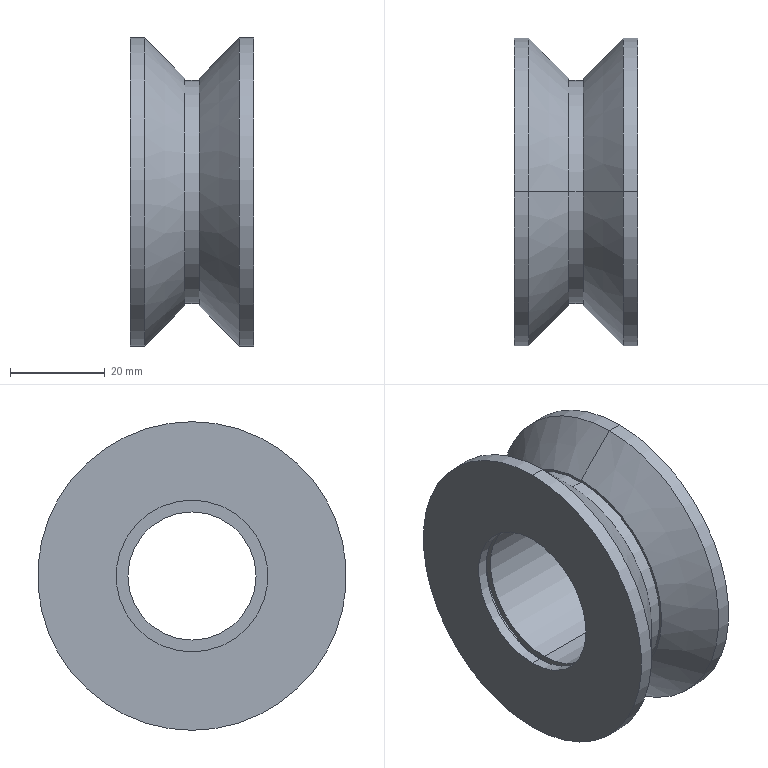Part | STEP file | X77-03304 | 1 solid | 25 faces | box 26 x 65 x 65 mm | volume 47550 mm3 | cylinder 14 | plane 7 | cone 4 | commonest cylinder face diameters 32 x4 65 x4 27 x2 34.6 x2 47 x2
STEP:
#1=CARTESIAN_POINT('',(10.752,77.79,23.5));
#2=VERTEX_POINT('',#1);
#3=CARTESIAN_POINT('',(10.752,77.79,-23.5));
#4=VERTEX_POINT('',#3);
#5=CARTESIAN_POINT('',(10.752,77.79,0.));
#6=DIRECTION('',(-1.,0.,0.));
#7=DIRECTION('',(0.,0.,1.));
#8=AXIS2_PLACEMENT_3D('',#5,#6,#7);
#9=CIRCLE('',#8,23.5);
#10=EDGE_CURVE('',#2,#4,#9,.T.);
#11=ORIENTED_EDGE('',*,*,#10,.T.);
#12=CARTESIAN_POINT('',(7.752,77.79,-23.5));
#13=VERTEX_POINT('',#12);
#14=CARTESIAN_POINT('',(-1000.,77.79,-23.5));
#15=DIRECTION('',(-1.,0.,0.));
#16=VECTOR('',#15,1000.);
#17=LINE('',#14,#16);
#18=EDGE_CURVE('',#4,#13,#17,.T.);
#19=ORIENTED_EDGE('',*,*,#18,.T.);
#20=CARTESIAN_POINT('',(7.752,77.79,23.5));
#21=VERTEX_POINT('',#20);
#22=CARTESIAN_POINT('',(7.752,77.79,0.));
#23=DIRECTION('',(-1.,0.,0.));
#24=DIRECTION('',(0.,0.,1.));
#25=AXIS2_PLACEMENT_3D('',#22,#23,#24);
#26=CIRCLE('',#25,23.5);
#27=EDGE_CURVE('',#21,#13,#26,.T.);
#28=ORIENTED_EDGE('',*,*,#27,.F.);
#29=CARTESIAN_POINT('',(-1000.,77.79,23.5));
#30=DIRECTION('',(-1.,0.,0.));
#31=VECTOR('',#30,1000.);
#32=LINE('',#29,#31);
#33=EDGE_CURVE('',#2,#21,#32,.T.);
#34=ORIENTED_EDGE('',*,*,#33,.F.);
#35=EDGE_LOOP('',(#11,#19,#28,#34));
#36=FACE_OUTER_BOUND('',#35,.T.);
#37=CARTESIAN_POINT('',(-1000.,77.79,0.));
#38=DIRECTION('',(-1.,0.,0.));
#39=DIRECTION('',(0.,0.,1.));
#40=AXIS2_PLACEMENT_3D('',#37,#38,#39);
#41=CYLINDRICAL_SURFACE('',#40,23.5);
#42=ADVANCED_FACE('',(#36),#41,.T.);
#43=CARTESIAN_POINT('',(7.752,77.79,24.));
#44=VERTEX_POINT('',#43);
#45=CARTESIAN_POINT('',(7.752,77.79,-24.));
#46=VERTEX_POINT('',#45);
#47=CARTESIAN_POINT('',(7.752,77.79,0.));
#48=DIRECTION('',(-1.,0.,0.));
#49=DIRECTION('',(0.,0.,1.));
#50=AXIS2_PLACEMENT_3D('',#47,#48,#49);
#51=CIRCLE('',#50,24.);
#52=EDGE_CURVE('',#44,#46,#51,.T.);
#53=ORIENTED_EDGE('',*,*,#52,.T.);
#54=CARTESIAN_POINT('',(-0.7476,77.79,-32.5));
#55=VERTEX_POINT('',#54);
#56=CARTESIAN_POINT('',(7.752,77.79,-24.));
#57=DIRECTION('',(-0.7071,0.,-0.7071));
#58=VECTOR('',#57,1000.);
#59=LINE('',#56,#58);
#60=EDGE_CURVE('',#46,#55,#59,.T.);
#61=ORIENTED_EDGE('',*,*,#60,.T.);
#62=CARTESIAN_POINT('',(-0.7476,77.79,32.5));
#63=VERTEX_POINT('',#62);
#64=CARTESIAN_POINT('',(-0.7476,77.79,0.));
#65=DIRECTION('',(-1.,0.,0.));
#66=DIRECTION('',(0.,0.,1.));
#67=AXIS2_PLACEMENT_3D('',#64,#65,#66);
#68=CIRCLE('',#67,32.5);
#69=EDGE_CURVE('',#63,#55,#68,.T.);
#70=ORIENTED_EDGE('',*,*,#69,.F.);
#71=CARTESIAN_POINT('',(7.752,77.79,24.));
#72=DIRECTION('',(-0.7071,0.,0.7071));
#73=VECTOR('',#72,1000.);
#74=LINE('',#71,#73);
#75=EDGE_CURVE('',#44,#63,#74,.T.);
#76=ORIENTED_EDGE('',*,*,#75,.F.);
#77=EDGE_LOOP('',(#53,#61,#70,#76));
#78=FACE_OUTER_BOUND('',#77,.T.);
#79=CARTESIAN_POINT('',(7.752,77.79,0.));
#80=DIRECTION('',(-1.,0.,0.));
#81=DIRECTION('',(0.,0.,1.));
#82=AXIS2_PLACEMENT_3D('',#79,#80,#81);
#83=CONICAL_SURFACE('',#82,24.,0.7854);
#84=ADVANCED_FACE('',(#78),#83,.T.);
#85=ORIENTED_EDGE('',*,*,#69,.T.);
#86=CARTESIAN_POINT('',(-3.748,77.79,-32.5));
#87=VERTEX_POINT('',#86);
#88=CARTESIAN_POINT('',(-1000.,77.79,-32.5));
#89=DIRECTION('',(-1.,0.,0.));
#90=VECTOR('',#89,1000.);
#91=LINE('',#88,#90);
#92=EDGE_CURVE('',#55,#87,#91,.T.);
#93=ORIENTED_EDGE('',*,*,#92,.T.);
#94=CARTESIAN_POINT('',(-3.748,77.79,32.5));
#95=VERTEX_POINT('',#94);
#96=CARTESIAN_POINT('',(-3.748,77.79,0.));
#97=DIRECTION('',(-1.,0.,0.));
#98=DIRECTION('',(0.,0.,1.));
#99=AXIS2_PLACEMENT_3D('',#96,#97,#98);
#100=CIRCLE('',#99,32.5);
#101=EDGE_CURVE('',#95,#87,#100,.T.);
#102=ORIENTED_EDGE('',*,*,#101,.F.);
#103=CARTESIAN_POINT('',(-1000.,77.79,32.5));
#104=DIRECTION('',(-1.,0.,0.));
#105=VECTOR('',#104,1000.);
#106=LINE('',#103,#105);
#107=EDGE_CURVE('',#63,#95,#106,.T.);
#108=ORIENTED_EDGE('',*,*,#107,.F.);
#109=EDGE_LOOP('',(#85,#93,#102,#108));
#110=FACE_OUTER_BOUND('',#109,.T.);
#111=CARTESIAN_POINT('',(-1000.,77.79,0.));
#112=DIRECTION('',(-1.,0.,0.));
#113=DIRECTION('',(0.,0.,1.));
#114=AXIS2_PLACEMENT_3D('',#111,#112,#113);
#115=CYLINDRICAL_SURFACE('',#114,32.5);
#116=ADVANCED_FACE('',(#110),#115,.T.);
#117=CARTESIAN_POINT('',(-1.548,77.79,-16.));
#118=VERTEX_POINT('',#117);
#119=CARTESIAN_POINT('',(-1.548,77.79,16.));
#120=VERTEX_POINT('',#119);
#121=CARTESIAN_POINT('',(-1.548,77.79,0.));
#122=DIRECTION('',(-1.,0.,0.));
#123=DIRECTION('',(0.,0.,1.));
#124=AXIS2_PLACEMENT_3D('',#121,#122,#123);
#125=CIRCLE('',#124,16.);
#126=EDGE_CURVE('',#118,#120,#125,.T.);
#127=ORIENTED_EDGE('',*,*,#126,.F.);
#128=CARTESIAN_POINT('',(-3.748,77.79,-16.));
#129=VERTEX_POINT('',#128);
#130=CARTESIAN_POINT('',(-1000.,77.79,-16.));
#131=DIRECTION('',(-1.,0.,0.));
#132=VECTOR('',#131,1000.);
#133=LINE('',#130,#132);
#134=EDGE_CURVE('',#118,#129,#133,.T.);
#135=ORIENTED_EDGE('',*,*,#134,.T.);
#136=CARTESIAN_POINT('',(-3.748,77.79,16.));
#137=VERTEX_POINT('',#136);
#138=CARTESIAN_POINT('',(-3.748,77.79,0.));
#139=DIRECTION('',(-1.,0.,0.));
#140=DIRECTION('',(0.,0.,1.));
#141=AXIS2_PLACEMENT_3D('',#138,#139,#140);
#142=CIRCLE('',#141,16.);
#143=EDGE_CURVE('',#129,#137,#142,.T.);
#144=ORIENTED_EDGE('',*,*,#143,.T.);
#145=CARTESIAN_POINT('',(-1000.,77.79,16.));
#146=DIRECTION('',(-1.,0.,0.));
#147=VECTOR('',#146,1000.);
#148=LINE('',#145,#147);
#149=EDGE_CURVE('',#120,#137,#148,.T.);
#150=ORIENTED_EDGE('',*,*,#149,.F.);
#151=EDGE_LOOP('',(#127,#135,#144,#150));
#152=FACE_OUTER_BOUND('',#151,.T.);
#153=CARTESIAN_POINT('',(-1000.,77.79,0.));
#154=DIRECTION('',(-1.,0.,0.));
#155=DIRECTION('',(0.,0.,1.));
#156=AXIS2_PLACEMENT_3D('',#153,#154,#155);
#157=CYLINDRICAL_SURFACE('',#156,16.);
#158=ADVANCED_FACE('',(#152),#157,.F.);
#159=CARTESIAN_POINT('',(-0.2476,77.79,-17.3));
#160=VERTEX_POINT('',#159);
#161=CARTESIAN_POINT('',(-0.2476,77.79,17.3));
#162=VERTEX_POINT('',#161);
#163=CARTESIAN_POINT('',(-0.2476,77.79,0.));
#164=DIRECTION('',(-1.,0.,0.));
#165=DIRECTION('',(0.,0.,1.));
#166=AXIS2_PLACEMENT_3D('',#163,#164,#165);
#167=CIRCLE('',#166,17.3);
#168=EDGE_CURVE('',#160,#162,#167,.T.);
#169=ORIENTED_EDGE('',*,*,#168,.F.);
#170=CARTESIAN_POINT('',(-1.548,77.79,-17.3));
#171=VERTEX_POINT('',#170);
#172=CARTESIAN_POINT('',(-1000.,77.79,-17.3));
#173=DIRECTION('',(-1.,0.,0.));
#174=VECTOR('',#173,1000.);
#175=LINE('',#172,#174);
#176=EDGE_CURVE('',#160,#171,#175,.T.);
#177=ORIENTED_EDGE('',*,*,#176,.T.);
#178=CARTESIAN_POINT('',(-1.548,77.79,17.3));
#179=VERTEX_POINT('',#178);
#180=CARTESIAN_POINT('',(-1.548,77.79,0.));
#181=DIRECTION('',(-1.,0.,0.));
#182=DIRECTION('',(0.,0.,1.));
#183=AXIS2_PLACEMENT_3D('',#180,#181,#182);
#184=CIRCLE('',#183,17.3);
#185=EDGE_CURVE('',#171,#179,#184,.T.);
#186=ORIENTED_EDGE('',*,*,#185,.T.);
#187=CARTESIAN_POINT('',(-1000.,77.79,17.3));
#188=DIRECTION('',(-1.,0.,0.));
#189=VECTOR('',#188,1000.);
#190=LINE('',#187,#189);
#191=EDGE_CURVE('',#162,#179,#190,.T.);
#192=ORIENTED_EDGE('',*,*,#191,.F.);
#193=EDGE_LOOP('',(#169,#177,#186,#192));
#194=FACE_OUTER_BOUND('',#193,.T.);
#195=CARTESIAN_POINT('',(-1000.,77.79,0.));
#196=DIRECTION('',(-1.,0.,0.));
#197=DIRECTION('',(0.,0.,1.));
#198=AXIS2_PLACEMENT_3D('',#195,#196,#197);
#199=CYLINDRICAL_SURFACE('',#198,17.3);
#200=ADVANCED_FACE('',(#194),#199,.F.);
#201=CARTESIAN_POINT('',(19.752,77.79,-16.));
#202=VERTEX_POINT('',#201);
#203=CARTESIAN_POINT('',(19.752,77.79,16.));
#204=VERTEX_POINT('',#203);
#205=CARTESIAN_POINT('',(19.752,77.79,0.));
#206=DIRECTION('',(-1.,0.,0.));
#207=DIRECTION('',(0.,0.,1.));
#208=AXIS2_PLACEMENT_3D('',#205,#206,#207);
#209=CIRCLE('',#208,16.);
#210=EDGE_CURVE('',#202,#204,#209,.T.);
#211=ORIENTED_EDGE('',*,*,#210,.F.);
#212=CARTESIAN_POINT('',(-0.2476,77.79,-16.));
#213=VERTEX_POINT('',#212);
#214=CARTESIAN_POINT('',(-1000.,77.79,-16.));
#215=DIRECTION('',(-1.,0.,0.));
#216=VECTOR('',#215,1000.);
#217=LINE('',#214,#216);
#218=EDGE_CURVE('',#202,#213,#217,.T.);
#219=ORIENTED_EDGE('',*,*,#218,.T.);
#220=CARTESIAN_POINT('',(-0.2476,77.79,16.));
#221=VERTEX_POINT('',#220);
#222=CARTESIAN_POINT('',(-0.2476,77.79,0.));
#223=DIRECTION('',(-1.,0.,0.));
#224=DIRECTION('',(0.,0.,1.));
#225=AXIS2_PLACEMENT_3D('',#222,#223,#224);
#226=CIRCLE('',#225,16.);
#227=EDGE_CURVE('',#213,#221,#226,.T.);
#228=ORIENTED_EDGE('',*,*,#227,.T.);
#229=CARTESIAN_POINT('',(-1000.,77.79,16.));
#230=DIRECTION('',(-1.,0.,0.));
#231=VECTOR('',#230,1000.);
#232=LINE('',#229,#231);
#233=EDGE_CURVE('',#204,#221,#232,.T.);
#234=ORIENTED_EDGE('',*,*,#233,.F.);
#235=EDGE_LOOP('',(#211,#219,#228,#234));
#236=FACE_OUTER_BOUND('',#235,.T.);
#237=CARTESIAN_POINT('',(-1000.,77.79,0.));
#238=DIRECTION('',(-1.,0.,0.));
#239=DIRECTION('',(0.,0.,1.));
#240=AXIS2_PLACEMENT_3D('',#237,#238,#239);
#241=CYLINDRICAL_SURFACE('',#240,16.);
#242=ADVANCED_FACE('',(#236),#241,.F.);
#243=CARTESIAN_POINT('',(22.252,77.79,-13.5));
#244=VERTEX_POINT('',#243);
#245=CARTESIAN_POINT('',(22.252,77.79,13.5));
#246=VERTEX_POINT('',#245);
#247=CARTESIAN_POINT('',(22.252,77.79,0.));
#248=DIRECTION('',(-1.,0.,0.));
#249=DIRECTION('',(0.,0.,1.));
#250=AXIS2_PLACEMENT_3D('',#247,#248,#249);
#251=CIRCLE('',#250,13.5);
#252=EDGE_CURVE('',#244,#246,#251,.T.);
#253=ORIENTED_EDGE('',*,*,#252,.F.);
#254=CARTESIAN_POINT('',(19.752,77.79,-13.5));
#255=VERTEX_POINT('',#254);
#256=CARTESIAN_POINT('',(-1000.,77.79,-13.5));
#257=DIRECTION('',(-1.,0.,0.));
#258=VECTOR('',#257,1000.);
#259=LINE('',#256,#258);
#260=EDGE_CURVE('',#244,#255,#259,.T.);
#261=ORIENTED_EDGE('',*,*,#260,.T.);
#262=CARTESIAN_POINT('',(19.752,77.79,13.5));
#263=VERTEX_POINT('',#262);
#264=CARTESIAN_POINT('',(19.752,77.79,0.));
#265=DIRECTION('',(-1.,0.,0.));
#266=DIRECTION('',(0.,0.,1.));
#267=AXIS2_PLACEMENT_3D('',#264,#265,#266);
#268=CIRCLE('',#267,13.5);
#269=EDGE_CURVE('',#255,#263,#268,.T.);
#270=ORIENTED_EDGE('',*,*,#269,.T.);
#271=CARTESIAN_POINT('',(-1000.,77.79,13.5));
#272=DIRECTION('',(-1.,0.,0.));
#273=VECTOR('',#272,1000.);
#274=LINE('',#271,#273);
#275=EDGE_CURVE('',#246,#263,#274,.T.);
#276=ORIENTED_EDGE('',*,*,#275,.F.);
#277=EDGE_LOOP('',(#253,#261,#270,#276));
#278=FACE_OUTER_BOUND('',#277,.T.);
#279=CARTESIAN_POINT('',(-1000.,77.79,0.));
#280=DIRECTION('',(-1.,0.,0.));
#281=DIRECTION('',(0.,0.,1.));
#282=AXIS2_PLACEMENT_3D('',#279,#280,#281);
#283=CYLINDRICAL_SURFACE('',#282,13.5);
#284=ADVANCED_FACE('',(#278),#283,.F.);
#285=CARTESIAN_POINT('',(22.252,77.79,32.5));
#286=VERTEX_POINT('',#285);
#287=CARTESIAN_POINT('',(22.252,77.79,-32.5));
#288=VERTEX_POINT('',#287);
#289=CARTESIAN_POINT('',(22.252,77.79,0.));
#290=DIRECTION('',(-1.,0.,0.));
#291=DIRECTION('',(0.,0.,1.));
#292=AXIS2_PLACEMENT_3D('',#289,#290,#291);
#293=CIRCLE('',#292,32.5);
#294=EDGE_CURVE('',#286,#288,#293,.T.);
#295=ORIENTED_EDGE('',*,*,#294,.T.);
#296=CARTESIAN_POINT('',(19.252,77.79,-32.5));
#297=VERTEX_POINT('',#296);
#298=CARTESIAN_POINT('',(-1000.,77.79,-32.5));
#299=DIRECTION('',(-1.,0.,0.));
#300=VECTOR('',#299,1000.);
#301=LINE('',#298,#300);
#302=EDGE_CURVE('',#288,#297,#301,.T.);
#303=ORIENTED_EDGE('',*,*,#302,.T.);
#304=CARTESIAN_POINT('',(19.252,77.79,32.5));
#305=VERTEX_POINT('',#304);
#306=CARTESIAN_POINT('',(19.252,77.79,0.));
#307=DIRECTION('',(-1.,0.,0.));
#308=DIRECTION('',(0.,0.,1.));
#309=AXIS2_PLACEMENT_3D('',#306,#307,#308);
#310=CIRCLE('',#309,32.5);
#311=EDGE_CURVE('',#305,#297,#310,.T.);
#312=ORIENTED_EDGE('',*,*,#311,.F.);
#313=CARTESIAN_POINT('',(-1000.,77.79,32.5));
#314=DIRECTION('',(-1.,0.,0.));
#315=VECTOR('',#314,1000.);
#316=LINE('',#313,#315);
#317=EDGE_CURVE('',#286,#305,#316,.T.);
#318=ORIENTED_EDGE('',*,*,#317,.F.);
#319=EDGE_LOOP('',(#295,#303,#312,#318));
#320=FACE_OUTER_BOUND('',#319,.T.);
#321=CARTESIAN_POINT('',(-1000.,77.79,0.));
#322=DIRECTION('',(-1.,0.,0.));
#323=DIRECTION('',(0.,0.,1.));
#324=AXIS2_PLACEMENT_3D('',#321,#322,#323);
#325=CYLINDRICAL_SURFACE('',#324,32.5);
#326=ADVANCED_FACE('',(#320),#325,.T.);
#327=CARTESIAN_POINT('',(10.752,77.79,24.));
#328=VERTEX_POINT('',#327);
#329=CARTESIAN_POINT('',(10.752,77.79,-24.));
#330=VERTEX_POINT('',#329);
#331=CARTESIAN_POINT('',(10.752,77.79,0.));
#332=DIRECTION('',(-1.,0.,0.));
#333=DIRECTION('',(0.,0.,1.));
#334=AXIS2_PLACEMENT_3D('',#331,#332,#333);
#335=CIRCLE('',#334,24.);
#336=EDGE_CURVE('',#328,#330,#335,.T.);
#337=ORIENTED_EDGE('',*,*,#336,.F.);
#338=CARTESIAN_POINT('',(19.252,77.79,32.5));
#339=DIRECTION('',(0.7071,0.,0.7071));
#340=VECTOR('',#339,1000.);
#341=LINE('',#338,#340);
#342=EDGE_CURVE('',#328,#305,#341,.T.);
#343=ORIENTED_EDGE('',*,*,#342,.T.);
#344=ORIENTED_EDGE('',*,*,#311,.T.);
#345=CARTESIAN_POINT('',(19.252,77.79,-32.5));
#346=DIRECTION('',(0.7071,0.,-0.7071));
#347=VECTOR('',#346,1000.);
#348=LINE('',#345,#347);
#349=EDGE_CURVE('',#330,#297,#348,.T.);
#350=ORIENTED_EDGE('',*,*,#349,.F.);
#351=EDGE_LOOP('',(#337,#343,#344,#350));
#352=FACE_OUTER_BOUND('',#351,.T.);
#353=CARTESIAN_POINT('',(19.252,77.79,0.));
#354=DIRECTION('',(1.,0.,0.));
#355=DIRECTION('',(0.,0.,-1.));
#356=AXIS2_PLACEMENT_3D('',#353,#354,#355);
#357=CONICAL_SURFACE('',#356,32.5,0.7854);
#358=ADVANCED_FACE('',(#352),#357,.T.);
#359=ORIENTED_EDGE('',*,*,#342,.F.);
#360=CARTESIAN_POINT('',(10.752,77.79,0.));
#361=DIRECTION('',(-1.,0.,0.));
#362=DIRECTION('',(0.,0.,1.));
#363=AXIS2_PLACEMENT_3D('',#360,#361,#362);
#364=CIRCLE('',#363,24.);
#365=EDGE_CURVE('',#330,#328,#364,.T.);
#366=ORIENTED_EDGE('',*,*,#365,.F.);
#367=ORIENTED_EDGE('',*,*,#349,.T.);
#368=CARTESIAN_POINT('',(19.252,77.79,0.));
#369=DIRECTION('',(-1.,0.,0.));
#370=DIRECTION('',(0.,0.,1.));
#371=AXIS2_PLACEMENT_3D('',#368,#369,#370);
#372=CIRCLE('',#371,32.5);
#373=EDGE_CURVE('',#297,#305,#372,.T.);
#374=ORIENTED_EDGE('',*,*,#373,.T.);
#375=EDGE_LOOP('',(#359,#366,#367,#374));
#376=FACE_OUTER_BOUND('',#375,.T.);
#377=CARTESIAN_POINT('',(19.252,77.79,0.));
#378=DIRECTION('',(1.,0.,0.));
#379=DIRECTION('',(0.,0.,-1.));
#380=AXIS2_PLACEMENT_3D('',#377,#378,#379);
#381=CONICAL_SURFACE('',#380,32.5,0.7854);
#382=ADVANCED_FACE('',(#376),#381,.T.);
#383=ORIENTED_EDGE('',*,*,#302,.F.);
#384=CARTESIAN_POINT('',(22.252,77.79,0.));
#385=DIRECTION('',(-1.,0.,0.));
#386=DIRECTION('',(0.,0.,1.));
#387=AXIS2_PLACEMENT_3D('',#384,#385,#386);
#388=CIRCLE('',#387,32.5);
#389=EDGE_CURVE('',#288,#286,#388,.T.);
#390=ORIENTED_EDGE('',*,*,#389,.T.);
#391=ORIENTED_EDGE('',*,*,#317,.T.);
#392=ORIENTED_EDGE('',*,*,#373,.F.);
#393=EDGE_LOOP('',(#383,#390,#391,#392));
#394=FACE_OUTER_BOUND('',#393,.T.);
#395=CARTESIAN_POINT('',(-1000.,77.79,0.));
#396=DIRECTION('',(-1.,0.,0.));
#397=DIRECTION('',(0.,0.,1.));
#398=AXIS2_PLACEMENT_3D('',#395,#396,#397);
#399=CYLINDRICAL_SURFACE('',#398,32.5);
#400=ADVANCED_FACE('',(#394),#399,.T.);
#401=ORIENTED_EDGE('',*,*,#294,.F.);
#402=ORIENTED_EDGE('',*,*,#389,.F.);
#403=EDGE_LOOP('',(#401,#402));
#404=FACE_OUTER_BOUND('',#403,.T.);
#405=CARTESIAN_POINT('',(22.252,77.79,0.));
#406=DIRECTION('',(-1.,0.,0.));
#407=DIRECTION('',(0.,0.,1.));
#408=AXIS2_PLACEMENT_3D('',#405,#406,#407);
#409=CIRCLE('',#408,13.5);
#410=EDGE_CURVE('',#246,#244,#409,.T.);
#411=ORIENTED_EDGE('',*,*,#410,.T.);
#412=ORIENTED_EDGE('',*,*,#252,.T.);
#413=EDGE_LOOP('',(#411,#412));
#414=FACE_BOUND('',#413,.T.);
#415=CARTESIAN_POINT('',(22.252,110.29,0.));
#416=DIRECTION('',(-1.,0.,0.));
#417=DIRECTION('',(0.,0.,1.));
#418=AXIS2_PLACEMENT_3D('',#415,#416,#417);
#419=PLANE('',#418);
#420=ADVANCED_FACE('',(#404,#414),#419,.F.);
#421=ORIENTED_EDGE('',*,*,#260,.F.);
#422=ORIENTED_EDGE('',*,*,#410,.F.);
#423=ORIENTED_EDGE('',*,*,#275,.T.);
#424=CARTESIAN_POINT('',(19.752,77.79,0.));
#425=DIRECTION('',(-1.,0.,0.));
#426=DIRECTION('',(0.,0.,1.));
#427=AXIS2_PLACEMENT_3D('',#424,#425,#426);
#428=CIRCLE('',#427,13.5);
#429=EDGE_CURVE('',#263,#255,#428,.T.);
#430=ORIENTED_EDGE('',*,*,#429,.T.);
#431=EDGE_LOOP('',(#421,#422,#423,#430));
#432=FACE_OUTER_BOUND('',#431,.T.);
#433=CARTESIAN_POINT('',(-1000.,77.79,0.));
#434=DIRECTION('',(-1.,0.,0.));
#435=DIRECTION('',(0.,0.,1.));
#436=AXIS2_PLACEMENT_3D('',#433,#434,#435);
#437=CYLINDRICAL_SURFACE('',#436,13.5);
#438=ADVANCED_FACE('',(#432),#437,.F.);
#439=ORIENTED_EDGE('',*,*,#429,.F.);
#440=ORIENTED_EDGE('',*,*,#269,.F.);
#441=EDGE_LOOP('',(#439,#440));
#442=FACE_BOUND('',#441,.T.);
#443=CARTESIAN_POINT('',(19.752,77.79,0.));
#444=DIRECTION('',(-1.,0.,0.));
#445=DIRECTION('',(0.,0.,1.));
#446=AXIS2_PLACEMENT_3D('',#443,#444,#445);
#447=CIRCLE('',#446,16.);
#448=EDGE_CURVE('',#204,#202,#447,.T.);
#449=ORIENTED_EDGE('',*,*,#448,.T.);
#450=ORIENTED_EDGE('',*,*,#210,.T.);
#451=EDGE_LOOP('',(#449,#450));
#452=FACE_OUTER_BOUND('',#451,.T.);
#453=CARTESIAN_POINT('',(19.752,91.29,0.));
#454=DIRECTION('',(1.,0.,0.));
#455=DIRECTION('',(0.,0.,-1.));
#456=AXIS2_PLACEMENT_3D('',#453,#454,#455);
#457=PLANE('',#456);
#458=ADVANCED_FACE('',(#442,#452),#457,.F.);
#459=ORIENTED_EDGE('',*,*,#218,.F.);
#460=ORIENTED_EDGE('',*,*,#448,.F.);
#461=ORIENTED_EDGE('',*,*,#233,.T.);
#462=CARTESIAN_POINT('',(-0.2476,77.79,0.));
#463=DIRECTION('',(-1.,0.,0.));
#464=DIRECTION('',(0.,0.,1.));
#465=AXIS2_PLACEMENT_3D('',#462,#463,#464);
#466=CIRCLE('',#465,16.);
#467=EDGE_CURVE('',#221,#213,#466,.T.);
#468=ORIENTED_EDGE('',*,*,#467,.T.);
#469=EDGE_LOOP('',(#459,#460,#461,#468));
#470=FACE_OUTER_BOUND('',#469,.T.);
#471=CARTESIAN_POINT('',(-1000.,77.79,0.));
#472=DIRECTION('',(-1.,0.,0.));
#473=DIRECTION('',(0.,0.,1.));
#474=AXIS2_PLACEMENT_3D('',#471,#472,#473);
#475=CYLINDRICAL_SURFACE('',#474,16.);
#476=ADVANCED_FACE('',(#470),#475,.F.);
#477=ORIENTED_EDGE('',*,*,#467,.F.);
#478=ORIENTED_EDGE('',*,*,#227,.F.);
#479=EDGE_LOOP('',(#477,#478));
#480=FACE_BOUND('',#479,.T.);
#481=CARTESIAN_POINT('',(-0.2476,77.79,0.));
#482=DIRECTION('',(-1.,0.,0.));
#483=DIRECTION('',(0.,0.,1.));
#484=AXIS2_PLACEMENT_3D('',#481,#482,#483);
#485=CIRCLE('',#484,17.3);
#486=EDGE_CURVE('',#162,#160,#485,.T.);
#487=ORIENTED_EDGE('',*,*,#486,.T.);
#488=ORIENTED_EDGE('',*,*,#168,.T.);
#489=EDGE_LOOP('',(#487,#488));
#490=FACE_OUTER_BOUND('',#489,.T.);
#491=CARTESIAN_POINT('',(-0.2476,95.09,0.));
#492=DIRECTION('',(1.,0.,0.));
#493=DIRECTION('',(0.,0.,-1.));
#494=AXIS2_PLACEMENT_3D('',#491,#492,#493);
#495=PLANE('',#494);
#496=ADVANCED_FACE('',(#480,#490),#495,.F.);
#497=ORIENTED_EDGE('',*,*,#176,.F.);
#498=ORIENTED_EDGE('',*,*,#486,.F.);
#499=ORIENTED_EDGE('',*,*,#191,.T.);
#500=CARTESIAN_POINT('',(-1.548,77.79,0.));
#501=DIRECTION('',(-1.,0.,0.));
#502=DIRECTION('',(0.,0.,1.));
#503=AXIS2_PLACEMENT_3D('',#500,#501,#502);
#504=CIRCLE('',#503,17.3);
#505=EDGE_CURVE('',#179,#171,#504,.T.);
#506=ORIENTED_EDGE('',*,*,#505,.T.);
#507=EDGE_LOOP('',(#497,#498,#499,#506));
#508=FACE_OUTER_BOUND('',#507,.T.);
#509=CARTESIAN_POINT('',(-1000.,77.79,0.));
#510=DIRECTION('',(-1.,0.,0.));
#511=DIRECTION('',(0.,0.,1.));
#512=AXIS2_PLACEMENT_3D('',#509,#510,#511);
#513=CYLINDRICAL_SURFACE('',#512,17.3);
#514=ADVANCED_FACE('',(#508),#513,.F.);
#515=ORIENTED_EDGE('',*,*,#505,.F.);
#516=ORIENTED_EDGE('',*,*,#185,.F.);
#517=EDGE_LOOP('',(#515,#516));
#518=FACE_OUTER_BOUND('',#517,.T.);
#519=CARTESIAN_POINT('',(-1.548,77.79,0.));
#520=DIRECTION('',(-1.,0.,0.));
#521=DIRECTION('',(0.,0.,1.));
#522=AXIS2_PLACEMENT_3D('',#519,#520,#521);
#523=CIRCLE('',#522,16.);
#524=EDGE_CURVE('',#120,#118,#523,.T.);
#525=ORIENTED_EDGE('',*,*,#524,.T.);
#526=ORIENTED_EDGE('',*,*,#126,.T.);
#527=EDGE_LOOP('',(#525,#526));
#528=FACE_BOUND('',#527,.T.);
#529=CARTESIAN_POINT('',(-1.548,93.79,0.));
#530=DIRECTION('',(-1.,0.,0.));
#531=DIRECTION('',(0.,0.,1.));
#532=AXIS2_PLACEMENT_3D('',#529,#530,#531);
#533=PLANE('',#532);
#534=ADVANCED_FACE('',(#518,#528),#533,.F.);
#535=ORIENTED_EDGE('',*,*,#134,.F.);
#536=ORIENTED_EDGE('',*,*,#524,.F.);
#537=ORIENTED_EDGE('',*,*,#149,.T.);
#538=CARTESIAN_POINT('',(-3.748,77.79,0.));
#539=DIRECTION('',(-1.,0.,0.));
#540=DIRECTION('',(0.,0.,1.));
#541=AXIS2_PLACEMENT_3D('',#538,#539,#540);
#542=CIRCLE('',#541,16.);
#543=EDGE_CURVE('',#137,#129,#542,.T.);
#544=ORIENTED_EDGE('',*,*,#543,.T.);
#545=EDGE_LOOP('',(#535,#536,#537,#544));
#546=FACE_OUTER_BOUND('',#545,.T.);
#547=CARTESIAN_POINT('',(-1000.,77.79,0.));
#548=DIRECTION('',(-1.,0.,0.));
#549=DIRECTION('',(0.,0.,1.));
#550=AXIS2_PLACEMENT_3D('',#547,#548,#549);
#551=CYLINDRICAL_SURFACE('',#550,16.);
#552=ADVANCED_FACE('',(#546),#551,.F.);
#553=ORIENTED_EDGE('',*,*,#543,.F.);
#554=ORIENTED_EDGE('',*,*,#143,.F.);
#555=EDGE_LOOP('',(#553,#554));
#556=FACE_BOUND('',#555,.T.);
#557=ORIENTED_EDGE('',*,*,#101,.T.);
#558=CARTESIAN_POINT('',(-3.748,77.79,0.));
#559=DIRECTION('',(-1.,0.,0.));
#560=DIRECTION('',(0.,0.,1.));
#561=AXIS2_PLACEMENT_3D('',#558,#559,#560);
#562=CIRCLE('',#561,32.5);
#563=EDGE_CURVE('',#87,#95,#562,.T.);
#564=ORIENTED_EDGE('',*,*,#563,.T.);
#565=EDGE_LOOP('',(#557,#564));
#566=FACE_OUTER_BOUND('',#565,.T.);
#567=CARTESIAN_POINT('',(-3.748,110.29,0.));
#568=DIRECTION('',(1.,0.,0.));
#569=DIRECTION('',(0.,0.,-1.));
#570=AXIS2_PLACEMENT_3D('',#567,#568,#569);
#571=PLANE('',#570);
#572=ADVANCED_FACE('',(#556,#566),#571,.F.);
#573=ORIENTED_EDGE('',*,*,#92,.F.);
#574=CARTESIAN_POINT('',(-0.7476,77.79,0.));
#575=DIRECTION('',(-1.,0.,0.));
#576=DIRECTION('',(0.,0.,1.));
#577=AXIS2_PLACEMENT_3D('',#574,#575,#576);
#578=CIRCLE('',#577,32.5);
#579=EDGE_CURVE('',#55,#63,#578,.T.);
#580=ORIENTED_EDGE('',*,*,#579,.T.);
#581=ORIENTED_EDGE('',*,*,#107,.T.);
#582=ORIENTED_EDGE('',*,*,#563,.F.);
#583=EDGE_LOOP('',(#573,#580,#581,#582));
#584=FACE_OUTER_BOUND('',#583,.T.);
#585=CARTESIAN_POINT('',(-1000.,77.79,0.));
#586=DIRECTION('',(-1.,0.,0.));
#587=DIRECTION('',(0.,0.,1.));
#588=AXIS2_PLACEMENT_3D('',#585,#586,#587);
#589=CYLINDRICAL_SURFACE('',#588,32.5);
#590=ADVANCED_FACE('',(#584),#589,.T.);
#591=ORIENTED_EDGE('',*,*,#60,.F.);
#592=CARTESIAN_POINT('',(7.752,77.79,0.));
#593=DIRECTION('',(-1.,0.,0.));
#594=DIRECTION('',(0.,0.,1.));
#595=AXIS2_PLACEMENT_3D('',#592,#593,#594);
#596=CIRCLE('',#595,24.);
#597=EDGE_CURVE('',#46,#44,#596,.T.);
#598=ORIENTED_EDGE('',*,*,#597,.T.);
#599=ORIENTED_EDGE('',*,*,#75,.T.);
#600=ORIENTED_EDGE('',*,*,#579,.F.);
#601=EDGE_LOOP('',(#591,#598,#599,#600));
#602=FACE_OUTER_BOUND('',#601,.T.);
#603=CARTESIAN_POINT('',(7.752,77.79,0.));
#604=DIRECTION('',(-1.,0.,0.));
#605=DIRECTION('',(0.,0.,1.));
#606=AXIS2_PLACEMENT_3D('',#603,#604,#605);
#607=CONICAL_SURFACE('',#606,24.,0.7854);
#608=ADVANCED_FACE('',(#602),#607,.T.);
#609=ORIENTED_EDGE('',*,*,#52,.F.);
#610=ORIENTED_EDGE('',*,*,#597,.F.);
#611=EDGE_LOOP('',(#609,#610));
#612=FACE_OUTER_BOUND('',#611,.T.);
#613=ORIENTED_EDGE('',*,*,#27,.T.);
#614=CARTESIAN_POINT('',(7.752,77.79,0.));
#615=DIRECTION('',(-1.,0.,0.));
#616=DIRECTION('',(0.,0.,1.));
#617=AXIS2_PLACEMENT_3D('',#614,#615,#616);
#618=CIRCLE('',#617,23.5);
#619=EDGE_CURVE('',#13,#21,#618,.T.);
#620=ORIENTED_EDGE('',*,*,#619,.T.);
#621=EDGE_LOOP('',(#613,#620));
#622=FACE_BOUND('',#621,.T.);
#623=CARTESIAN_POINT('',(7.752,101.79,0.));
#624=DIRECTION('',(-1.,0.,0.));
#625=DIRECTION('',(0.,0.,1.));
#626=AXIS2_PLACEMENT_3D('',#623,#624,#625);
#627=PLANE('',#626);
#628=ADVANCED_FACE('',(#612,#622),#627,.F.);
#629=ORIENTED_EDGE('',*,*,#18,.F.);
#630=CARTESIAN_POINT('',(10.752,77.79,0.));
#631=DIRECTION('',(-1.,0.,0.));
#632=DIRECTION('',(0.,0.,1.));
#633=AXIS2_PLACEMENT_3D('',#630,#631,#632);
#634=CIRCLE('',#633,23.5);
#635=EDGE_CURVE('',#4,#2,#634,.T.);
#636=ORIENTED_EDGE('',*,*,#635,.T.);
#637=ORIENTED_EDGE('',*,*,#33,.T.);
#638=ORIENTED_EDGE('',*,*,#619,.F.);
#639=EDGE_LOOP('',(#629,#636,#637,#638));
#640=FACE_OUTER_BOUND('',#639,.T.);
#641=CARTESIAN_POINT('',(-1000.,77.79,0.));
#642=DIRECTION('',(-1.,0.,0.));
#643=DIRECTION('',(0.,0.,1.));
#644=AXIS2_PLACEMENT_3D('',#641,#642,#643);
#645=CYLINDRICAL_SURFACE('',#644,23.5);
#646=ADVANCED_FACE('',(#640),#645,.T.);
#647=ORIENTED_EDGE('',*,*,#10,.F.);
#648=ORIENTED_EDGE('',*,*,#635,.F.);
#649=EDGE_LOOP('',(#647,#648));
#650=FACE_BOUND('',#649,.T.);
#651=ORIENTED_EDGE('',*,*,#365,.T.);
#652=ORIENTED_EDGE('',*,*,#336,.T.);
#653=EDGE_LOOP('',(#651,#652));
#654=FACE_OUTER_BOUND('',#653,.T.);
#655=CARTESIAN_POINT('',(10.752,101.29,0.));
#656=DIRECTION('',(1.,0.,0.));
#657=DIRECTION('',(0.,0.,-1.));
#658=AXIS2_PLACEMENT_3D('',#655,#656,#657);
#659=PLANE('',#658);
#660=ADVANCED_FACE('',(#650,#654),#659,.F.);
#661=CLOSED_SHELL('',(#42,#84,#116,#158,#200,#242,#284,#326,#358,#382,#400,#420,#438,#458,#476,#496,#514,#534,#552,#572,#590,#608,#628,#646,#660));
#662=MANIFOLD_SOLID_BREP('',#661);
#663=CARTESIAN_POINT('',(0.,0.,0.));
#664=DIRECTION('',(0.,0.,1.));
#665=DIRECTION('',(1.,0.,0.));
#666=AXIS2_PLACEMENT_3D('',#663,#664,#665);
#667=(LENGTH_UNIT()NAMED_UNIT(*)SI_UNIT(.MILLI.,.METRE.));
#668=UNCERTAINTY_MEASURE_WITH_UNIT(LENGTH_MEASURE(0.00001),#667,'','');
#669=(NAMED_UNIT(*)PLANE_ANGLE_UNIT()SI_UNIT($,.RADIAN.));
#670=(NAMED_UNIT(*)SI_UNIT($,.STERADIAN.)SOLID_ANGLE_UNIT());
#671=(GEOMETRIC_REPRESENTATION_CONTEXT(3)GLOBAL_UNCERTAINTY_ASSIGNED_CONTEXT((#668))GLOBAL_UNIT_ASSIGNED_CONTEXT((#667,#669,#670))REPRESENTATION_CONTEXT('',''));
#672=ADVANCED_BREP_SHAPE_REPRESENTATION('',(#662,#666),#671);